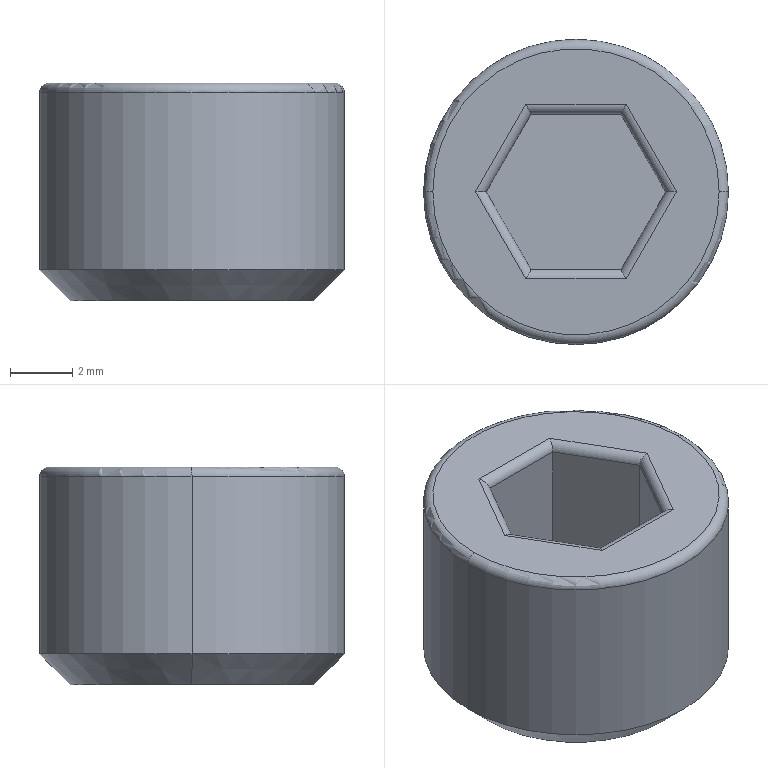Part | STEP file | P-015007 | 1 solid | 21 faces | box 9.8 x 9.8 x 7 mm | volume 415.303 mm3 | plane 9 | cylinder 8 | torus 2 | cone 2 | commonest cylinder face diameters 0.6 x6 9.8 x2